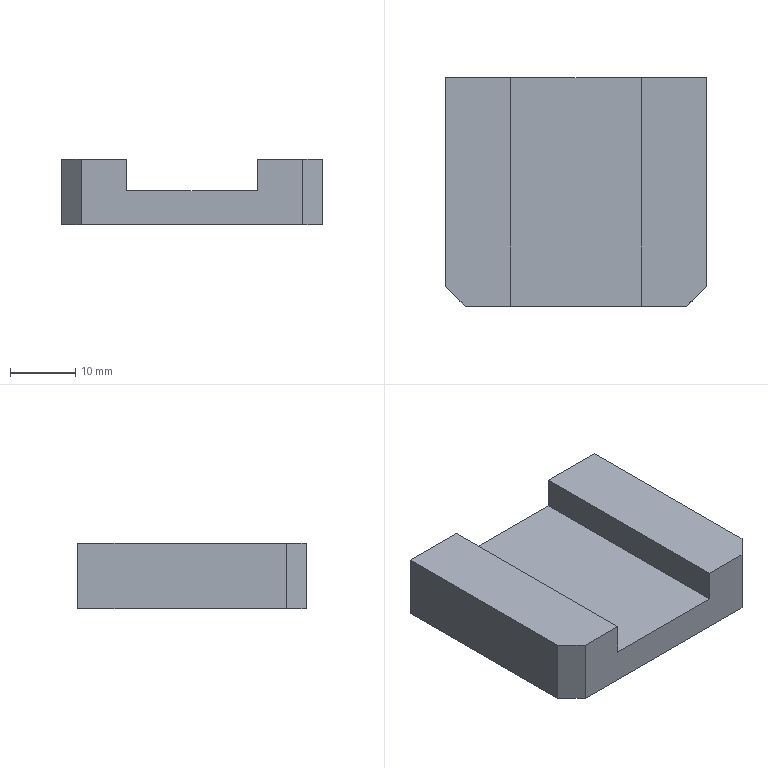Part | STEP file | PN_0017 | 1 solid | 12 faces | box 40 x 35 x 10 mm | volume 10550 mm3 | plane 12
STEP:
#1=CARTESIAN_POINT('',(0.,0.,0.));
#2=DIRECTION('',(0.,0.,1.));
#3=DIRECTION('',(1.,0.,0.));
#4=AXIS2_PLACEMENT_3D('',#1,#2,#3);
#5=CARTESIAN_POINT('',(10.,-17.5,10.));
#6=VERTEX_POINT('',#5);
#7=CARTESIAN_POINT('',(17.,-17.5,10.));
#8=VERTEX_POINT('',#7);
#9=CARTESIAN_POINT('',(-20.,-17.5,10.));
#10=DIRECTION('',(1.,0.,0.));
#11=VECTOR('',#10,1.);
#12=LINE('',#9,#11);
#13=CARTESIAN_POINT('',(20.,-17.5,10.));
#14=DIRECTION('',(0.,0.,1.));
#15=DIRECTION('',(1.,0.,0.));
#16=AXIS2_PLACEMENT_3D('',#13,#14,#15);
#17=PLANE('',#16);
#18=CARTESIAN_POINT('',(-40.,0.));
#19=DIRECTION('',(1.,0.));
#20=VECTOR('',#19,1.);
#21=LINE('',#18,#20);
#22=(GEOMETRIC_REPRESENTATION_CONTEXT(2)PARAMETRIC_REPRESENTATION_CONTEXT()REPRESENTATION_CONTEXT('',''));
#23=DEFINITIONAL_REPRESENTATION('',(#21),#22);
#24=PCURVE('',#17,#23);
#25=CARTESIAN_POINT('',(-20.,-17.5,10.));
#26=DIRECTION('',(0.,1.,0.));
#27=DIRECTION('',(0.,0.,1.));
#28=AXIS2_PLACEMENT_3D('',#25,#26,#27);
#29=PLANE('',#28);
#30=CARTESIAN_POINT('',(0.,0.));
#31=DIRECTION('',(0.,1.));
#32=VECTOR('',#31,1.);
#33=LINE('',#30,#32);
#34=(GEOMETRIC_REPRESENTATION_CONTEXT(2)PARAMETRIC_REPRESENTATION_CONTEXT()REPRESENTATION_CONTEXT('',''));
#35=DEFINITIONAL_REPRESENTATION('',(#33),#34);
#36=PCURVE('',#29,#35);
#37=SURFACE_CURVE('',#12,(#24,#36),.PCURVE_S1.);
#38=EDGE_CURVE('',#6,#8,#37,.T.);
#39=ORIENTED_EDGE('',*,*,#38,.T.);
#40=CARTESIAN_POINT('',(20.,-14.5,10.));
#41=VERTEX_POINT('',#40);
#42=CARTESIAN_POINT('',(18.5,-16.,10.));
#43=DIRECTION('',(0.7071,0.7071,0.));
#44=VECTOR('',#43,1.);
#45=LINE('',#42,#44);
#46=CARTESIAN_POINT('',(-1.5,1.5));
#47=DIRECTION('',(0.7071,0.7071));
#48=VECTOR('',#47,1.);
#49=LINE('',#46,#48);
#50=(GEOMETRIC_REPRESENTATION_CONTEXT(2)PARAMETRIC_REPRESENTATION_CONTEXT()REPRESENTATION_CONTEXT('',''));
#51=DEFINITIONAL_REPRESENTATION('',(#49),#50);
#52=PCURVE('',#17,#51);
#53=CARTESIAN_POINT('',(20.,-14.5,10.));
#54=DIRECTION('',(-0.7071,0.7071,0.));
#55=DIRECTION('',(-0.7071,-0.7071,0.));
#56=AXIS2_PLACEMENT_3D('',#53,#54,#55);
#57=PLANE('',#56);
#58=CARTESIAN_POINT('',(2.121,0.));
#59=DIRECTION('',(-1.,0.));
#60=VECTOR('',#59,1.);
#61=LINE('',#58,#60);
#62=(GEOMETRIC_REPRESENTATION_CONTEXT(2)PARAMETRIC_REPRESENTATION_CONTEXT()REPRESENTATION_CONTEXT('',''));
#63=DEFINITIONAL_REPRESENTATION('',(#61),#62);
#64=PCURVE('',#57,#63);
#65=SURFACE_CURVE('',#45,(#52,#64),.PCURVE_S1.);
#66=EDGE_CURVE('',#8,#41,#65,.T.);
#67=ORIENTED_EDGE('',*,*,#66,.T.);
#68=CARTESIAN_POINT('',(20.,17.5,10.));
#69=VERTEX_POINT('',#68);
#70=CARTESIAN_POINT('',(20.,17.5,10.));
#71=DIRECTION('',(0.,1.,0.));
#72=VECTOR('',#71,1.);
#73=LINE('',#70,#72);
#74=CARTESIAN_POINT('',(0.,35.));
#75=DIRECTION('',(0.,1.));
#76=VECTOR('',#75,1.);
#77=LINE('',#74,#76);
#78=(GEOMETRIC_REPRESENTATION_CONTEXT(2)PARAMETRIC_REPRESENTATION_CONTEXT()REPRESENTATION_CONTEXT('',''));
#79=DEFINITIONAL_REPRESENTATION('',(#77),#78);
#80=PCURVE('',#17,#79);
#81=CARTESIAN_POINT('',(20.,17.5,10.));
#82=DIRECTION('',(-1.,0.,0.));
#83=DIRECTION('',(0.,-1.,0.));
#84=AXIS2_PLACEMENT_3D('',#81,#82,#83);
#85=PLANE('',#84);
#86=CARTESIAN_POINT('',(0.,0.));
#87=DIRECTION('',(-1.,0.));
#88=VECTOR('',#87,1.);
#89=LINE('',#86,#88);
#90=(GEOMETRIC_REPRESENTATION_CONTEXT(2)PARAMETRIC_REPRESENTATION_CONTEXT()REPRESENTATION_CONTEXT('',''));
#91=DEFINITIONAL_REPRESENTATION('',(#89),#90);
#92=PCURVE('',#85,#91);
#93=SURFACE_CURVE('',#73,(#80,#92),.PCURVE_S1.);
#94=EDGE_CURVE('',#41,#69,#93,.T.);
#95=ORIENTED_EDGE('',*,*,#94,.T.);
#96=CARTESIAN_POINT('',(10.,17.5,10.));
#97=VERTEX_POINT('',#96);
#98=CARTESIAN_POINT('',(-20.,17.5,10.));
#99=DIRECTION('',(-1.,0.,0.));
#100=VECTOR('',#99,1.);
#101=LINE('',#98,#100);
#102=CARTESIAN_POINT('',(-40.,35.));
#103=DIRECTION('',(-1.,0.));
#104=VECTOR('',#103,1.);
#105=LINE('',#102,#104);
#106=(GEOMETRIC_REPRESENTATION_CONTEXT(2)PARAMETRIC_REPRESENTATION_CONTEXT()REPRESENTATION_CONTEXT('',''));
#107=DEFINITIONAL_REPRESENTATION('',(#105),#106);
#108=PCURVE('',#17,#107);
#109=CARTESIAN_POINT('',(-20.,17.5,10.));
#110=DIRECTION('',(0.,-1.,0.));
#111=DIRECTION('',(0.,0.,-1.));
#112=AXIS2_PLACEMENT_3D('',#109,#110,#111);
#113=PLANE('',#112);
#114=CARTESIAN_POINT('',(0.,0.));
#115=DIRECTION('',(0.,-1.));
#116=VECTOR('',#115,1.);
#117=LINE('',#114,#116);
#118=(GEOMETRIC_REPRESENTATION_CONTEXT(2)PARAMETRIC_REPRESENTATION_CONTEXT()REPRESENTATION_CONTEXT('',''));
#119=DEFINITIONAL_REPRESENTATION('',(#117),#118);
#120=PCURVE('',#113,#119);
#121=SURFACE_CURVE('',#101,(#108,#120),.PCURVE_S1.);
#122=EDGE_CURVE('',#69,#97,#121,.T.);
#123=ORIENTED_EDGE('',*,*,#122,.T.);
#124=CARTESIAN_POINT('',(10.,17.5,10.));
#125=DIRECTION('',(0.,1.,0.));
#126=VECTOR('',#125,1.);
#127=LINE('',#124,#126);
#128=CARTESIAN_POINT('',(-10.,35.));
#129=DIRECTION('',(0.,1.));
#130=VECTOR('',#129,1.);
#131=LINE('',#128,#130);
#132=(GEOMETRIC_REPRESENTATION_CONTEXT(2)PARAMETRIC_REPRESENTATION_CONTEXT()REPRESENTATION_CONTEXT('',''));
#133=DEFINITIONAL_REPRESENTATION('',(#131),#132);
#134=PCURVE('',#17,#133);
#135=CARTESIAN_POINT('',(10.,17.5,5.2));
#136=DIRECTION('',(1.,0.,0.));
#137=DIRECTION('',(0.,0.,-1.));
#138=AXIS2_PLACEMENT_3D('',#135,#136,#137);
#139=PLANE('',#138);
#140=CARTESIAN_POINT('',(-4.8,0.));
#141=DIRECTION('',(0.,1.));
#142=VECTOR('',#141,1.);
#143=LINE('',#140,#142);
#144=(GEOMETRIC_REPRESENTATION_CONTEXT(2)PARAMETRIC_REPRESENTATION_CONTEXT()REPRESENTATION_CONTEXT('',''));
#145=DEFINITIONAL_REPRESENTATION('',(#143),#144);
#146=PCURVE('',#139,#145);
#147=SURFACE_CURVE('',#127,(#134,#146),.PCURVE_S1.);
#148=EDGE_CURVE('',#6,#97,#147,.T.);
#149=ORIENTED_EDGE('',*,*,#148,.F.);
#150=EDGE_LOOP('',(#39,#67,#95,#123,#149));
#151=FACE_BOUND('',#150,.T.);
#152=ADVANCED_FACE('',(#151),#17,.T.);
#153=ORIENTED_EDGE('',*,*,#94,.F.);
#154=CARTESIAN_POINT('',(20.,-14.5,0.));
#155=VERTEX_POINT('',#154);
#156=CARTESIAN_POINT('',(20.,-14.5,10.));
#157=DIRECTION('',(0.,0.,-1.));
#158=VECTOR('',#157,1.);
#159=LINE('',#156,#158);
#160=CARTESIAN_POINT('',(32.,0.));
#161=DIRECTION('',(0.,-1.));
#162=VECTOR('',#161,1.);
#163=LINE('',#160,#162);
#164=(GEOMETRIC_REPRESENTATION_CONTEXT(2)PARAMETRIC_REPRESENTATION_CONTEXT()REPRESENTATION_CONTEXT('',''));
#165=DEFINITIONAL_REPRESENTATION('',(#163),#164);
#166=PCURVE('',#85,#165);
#167=CARTESIAN_POINT('',(0.,0.));
#168=DIRECTION('',(0.,-1.));
#169=VECTOR('',#168,1.);
#170=LINE('',#167,#169);
#171=(GEOMETRIC_REPRESENTATION_CONTEXT(2)PARAMETRIC_REPRESENTATION_CONTEXT()REPRESENTATION_CONTEXT('',''));
#172=DEFINITIONAL_REPRESENTATION('',(#170),#171);
#173=PCURVE('',#57,#172);
#174=SURFACE_CURVE('',#159,(#166,#173),.PCURVE_S1.);
#175=EDGE_CURVE('',#41,#155,#174,.T.);
#176=ORIENTED_EDGE('',*,*,#175,.T.);
#177=CARTESIAN_POINT('',(20.,17.5,0.));
#178=VERTEX_POINT('',#177);
#179=CARTESIAN_POINT('',(20.,17.5,0.));
#180=DIRECTION('',(0.,1.,0.));
#181=VECTOR('',#180,1.);
#182=LINE('',#179,#181);
#183=CARTESIAN_POINT('',(0.,-10.));
#184=DIRECTION('',(-1.,0.));
#185=VECTOR('',#184,1.);
#186=LINE('',#183,#185);
#187=(GEOMETRIC_REPRESENTATION_CONTEXT(2)PARAMETRIC_REPRESENTATION_CONTEXT()REPRESENTATION_CONTEXT('',''));
#188=DEFINITIONAL_REPRESENTATION('',(#186),#187);
#189=PCURVE('',#85,#188);
#190=CARTESIAN_POINT('',(20.,-17.5,0.));
#191=DIRECTION('',(0.,0.,1.));
#192=DIRECTION('',(1.,0.,0.));
#193=AXIS2_PLACEMENT_3D('',#190,#191,#192);
#194=PLANE('',#193);
#195=CARTESIAN_POINT('',(0.,35.));
#196=DIRECTION('',(0.,1.));
#197=VECTOR('',#196,1.);
#198=LINE('',#195,#197);
#199=(GEOMETRIC_REPRESENTATION_CONTEXT(2)PARAMETRIC_REPRESENTATION_CONTEXT()REPRESENTATION_CONTEXT('',''));
#200=DEFINITIONAL_REPRESENTATION('',(#198),#199);
#201=PCURVE('',#194,#200);
#202=SURFACE_CURVE('',#182,(#189,#201),.PCURVE_S1.);
#203=EDGE_CURVE('',#155,#178,#202,.T.);
#204=ORIENTED_EDGE('',*,*,#203,.T.);
#205=CARTESIAN_POINT('',(20.,17.5,10.));
#206=DIRECTION('',(0.,0.,-1.));
#207=VECTOR('',#206,1.);
#208=LINE('',#205,#207);
#209=CARTESIAN_POINT('',(0.,0.));
#210=DIRECTION('',(0.,-1.));
#211=VECTOR('',#210,1.);
#212=LINE('',#209,#211);
#213=(GEOMETRIC_REPRESENTATION_CONTEXT(2)PARAMETRIC_REPRESENTATION_CONTEXT()REPRESENTATION_CONTEXT('',''));
#214=DEFINITIONAL_REPRESENTATION('',(#212),#213);
#215=PCURVE('',#85,#214);
#216=CARTESIAN_POINT('',(0.,40.));
#217=DIRECTION('',(1.,0.));
#218=VECTOR('',#217,1.);
#219=LINE('',#216,#218);
#220=(GEOMETRIC_REPRESENTATION_CONTEXT(2)PARAMETRIC_REPRESENTATION_CONTEXT()REPRESENTATION_CONTEXT('',''));
#221=DEFINITIONAL_REPRESENTATION('',(#219),#220);
#222=PCURVE('',#113,#221);
#223=SURFACE_CURVE('',#208,(#215,#222),.PCURVE_S1.);
#224=EDGE_CURVE('',#69,#178,#223,.T.);
#225=ORIENTED_EDGE('',*,*,#224,.F.);
#226=EDGE_LOOP('',(#153,#176,#204,#225));
#227=FACE_BOUND('',#226,.T.);
#228=ADVANCED_FACE('',(#227),#85,.F.);
#229=CARTESIAN_POINT('',(10.,17.5,5.2));
#230=VERTEX_POINT('',#229);
#231=CARTESIAN_POINT('',(-10.,17.5,5.2));
#232=VERTEX_POINT('',#231);
#233=CARTESIAN_POINT('',(-10.,17.5,5.2));
#234=DIRECTION('',(-1.,0.,0.));
#235=VECTOR('',#234,1.);
#236=LINE('',#233,#235);
#237=CARTESIAN_POINT('',(4.8,10.));
#238=DIRECTION('',(0.,-1.));
#239=VECTOR('',#238,1.);
#240=LINE('',#237,#239);
#241=(GEOMETRIC_REPRESENTATION_CONTEXT(2)PARAMETRIC_REPRESENTATION_CONTEXT()REPRESENTATION_CONTEXT('',''));
#242=DEFINITIONAL_REPRESENTATION('',(#240),#241);
#243=PCURVE('',#113,#242);
#244=CARTESIAN_POINT('',(10.,-17.5,5.2));
#245=DIRECTION('',(0.,0.,1.));
#246=DIRECTION('',(1.,0.,0.));
#247=AXIS2_PLACEMENT_3D('',#244,#245,#246);
#248=PLANE('',#247);
#249=CARTESIAN_POINT('',(-20.,35.));
#250=DIRECTION('',(-1.,0.));
#251=VECTOR('',#250,1.);
#252=LINE('',#249,#251);
#253=(GEOMETRIC_REPRESENTATION_CONTEXT(2)PARAMETRIC_REPRESENTATION_CONTEXT()REPRESENTATION_CONTEXT('',''));
#254=DEFINITIONAL_REPRESENTATION('',(#252),#253);
#255=PCURVE('',#248,#254);
#256=SURFACE_CURVE('',#236,(#243,#255),.PCURVE_S1.);
#257=EDGE_CURVE('',#230,#232,#256,.T.);
#258=ORIENTED_EDGE('',*,*,#257,.F.);
#259=CARTESIAN_POINT('',(10.,17.5,5.2));
#260=DIRECTION('',(0.,0.,1.));
#261=VECTOR('',#260,1.);
#262=LINE('',#259,#261);
#263=CARTESIAN_POINT('',(4.8,30.));
#264=DIRECTION('',(-1.,0.));
#265=VECTOR('',#264,1.);
#266=LINE('',#263,#265);
#267=(GEOMETRIC_REPRESENTATION_CONTEXT(2)PARAMETRIC_REPRESENTATION_CONTEXT()REPRESENTATION_CONTEXT('',''));
#268=DEFINITIONAL_REPRESENTATION('',(#266),#267);
#269=PCURVE('',#113,#268);
#270=CARTESIAN_POINT('',(0.,0.));
#271=DIRECTION('',(-1.,0.));
#272=VECTOR('',#271,1.);
#273=LINE('',#270,#272);
#274=(GEOMETRIC_REPRESENTATION_CONTEXT(2)PARAMETRIC_REPRESENTATION_CONTEXT()REPRESENTATION_CONTEXT('',''));
#275=DEFINITIONAL_REPRESENTATION('',(#273),#274);
#276=PCURVE('',#139,#275);
#277=SURFACE_CURVE('',#262,(#269,#276),.PCURVE_S1.);
#278=EDGE_CURVE('',#230,#97,#277,.T.);
#279=ORIENTED_EDGE('',*,*,#278,.T.);
#280=ORIENTED_EDGE('',*,*,#122,.F.);
#281=ORIENTED_EDGE('',*,*,#224,.T.);
#282=CARTESIAN_POINT('',(-20.,17.5,0.));
#283=VERTEX_POINT('',#282);
#284=CARTESIAN_POINT('',(-20.,17.5,0.));
#285=DIRECTION('',(-1.,0.,0.));
#286=VECTOR('',#285,1.);
#287=LINE('',#284,#286);
#288=CARTESIAN_POINT('',(10.,0.));
#289=DIRECTION('',(0.,-1.));
#290=VECTOR('',#289,1.);
#291=LINE('',#288,#290);
#292=(GEOMETRIC_REPRESENTATION_CONTEXT(2)PARAMETRIC_REPRESENTATION_CONTEXT()REPRESENTATION_CONTEXT('',''));
#293=DEFINITIONAL_REPRESENTATION('',(#291),#292);
#294=PCURVE('',#113,#293);
#295=CARTESIAN_POINT('',(-40.,35.));
#296=DIRECTION('',(-1.,0.));
#297=VECTOR('',#296,1.);
#298=LINE('',#295,#297);
#299=(GEOMETRIC_REPRESENTATION_CONTEXT(2)PARAMETRIC_REPRESENTATION_CONTEXT()REPRESENTATION_CONTEXT('',''));
#300=DEFINITIONAL_REPRESENTATION('',(#298),#299);
#301=PCURVE('',#194,#300);
#302=SURFACE_CURVE('',#287,(#294,#301),.PCURVE_S1.);
#303=EDGE_CURVE('',#178,#283,#302,.T.);
#304=ORIENTED_EDGE('',*,*,#303,.T.);
#305=CARTESIAN_POINT('',(-20.,17.5,10.));
#306=VERTEX_POINT('',#305);
#307=CARTESIAN_POINT('',(-20.,17.5,10.));
#308=DIRECTION('',(0.,0.,-1.));
#309=VECTOR('',#308,1.);
#310=LINE('',#307,#309);
#311=CARTESIAN_POINT('',(0.,0.));
#312=DIRECTION('',(1.,0.));
#313=VECTOR('',#312,1.);
#314=LINE('',#311,#313);
#315=(GEOMETRIC_REPRESENTATION_CONTEXT(2)PARAMETRIC_REPRESENTATION_CONTEXT()REPRESENTATION_CONTEXT('',''));
#316=DEFINITIONAL_REPRESENTATION('',(#314),#315);
#317=PCURVE('',#113,#316);
#318=CARTESIAN_POINT('',(-20.,17.5,10.));
#319=DIRECTION('',(1.,0.,0.));
#320=DIRECTION('',(0.,1.,0.));
#321=AXIS2_PLACEMENT_3D('',#318,#319,#320);
#322=PLANE('',#321);
#323=CARTESIAN_POINT('',(0.,0.));
#324=DIRECTION('',(0.,-1.));
#325=VECTOR('',#324,1.);
#326=LINE('',#323,#325);
#327=(GEOMETRIC_REPRESENTATION_CONTEXT(2)PARAMETRIC_REPRESENTATION_CONTEXT()REPRESENTATION_CONTEXT('',''));
#328=DEFINITIONAL_REPRESENTATION('',(#326),#327);
#329=PCURVE('',#322,#328);
#330=SURFACE_CURVE('',#310,(#317,#329),.PCURVE_S1.);
#331=EDGE_CURVE('',#306,#283,#330,.T.);
#332=ORIENTED_EDGE('',*,*,#331,.F.);
#333=CARTESIAN_POINT('',(-10.,17.5,10.));
#334=VERTEX_POINT('',#333);
#335=CARTESIAN_POINT('',(-20.,17.5,10.));
#336=DIRECTION('',(-1.,0.,0.));
#337=VECTOR('',#336,1.);
#338=LINE('',#335,#337);
#339=CARTESIAN_POINT('',(0.,0.));
#340=DIRECTION('',(0.,-1.));
#341=VECTOR('',#340,1.);
#342=LINE('',#339,#341);
#343=(GEOMETRIC_REPRESENTATION_CONTEXT(2)PARAMETRIC_REPRESENTATION_CONTEXT()REPRESENTATION_CONTEXT('',''));
#344=DEFINITIONAL_REPRESENTATION('',(#342),#343);
#345=PCURVE('',#113,#344);
#346=CARTESIAN_POINT('',(20.,-17.5,10.));
#347=DIRECTION('',(0.,0.,1.));
#348=DIRECTION('',(1.,0.,0.));
#349=AXIS2_PLACEMENT_3D('',#346,#347,#348);
#350=PLANE('',#349);
#351=CARTESIAN_POINT('',(-40.,35.));
#352=DIRECTION('',(-1.,0.));
#353=VECTOR('',#352,1.);
#354=LINE('',#351,#353);
#355=(GEOMETRIC_REPRESENTATION_CONTEXT(2)PARAMETRIC_REPRESENTATION_CONTEXT()REPRESENTATION_CONTEXT('',''));
#356=DEFINITIONAL_REPRESENTATION('',(#354),#355);
#357=PCURVE('',#350,#356);
#358=SURFACE_CURVE('',#338,(#345,#357),.PCURVE_S1.);
#359=EDGE_CURVE('',#334,#306,#358,.T.);
#360=ORIENTED_EDGE('',*,*,#359,.F.);
#361=CARTESIAN_POINT('',(-10.,17.5,5.2));
#362=DIRECTION('',(0.,0.,1.));
#363=VECTOR('',#362,1.);
#364=LINE('',#361,#363);
#365=CARTESIAN_POINT('',(4.8,10.));
#366=DIRECTION('',(-1.,0.));
#367=VECTOR('',#366,1.);
#368=LINE('',#365,#367);
#369=(GEOMETRIC_REPRESENTATION_CONTEXT(2)PARAMETRIC_REPRESENTATION_CONTEXT()REPRESENTATION_CONTEXT('',''));
#370=DEFINITIONAL_REPRESENTATION('',(#368),#369);
#371=PCURVE('',#113,#370);
#372=CARTESIAN_POINT('',(-10.,17.5,5.2));
#373=DIRECTION('',(-1.,0.,0.));
#374=DIRECTION('',(0.,0.,1.));
#375=AXIS2_PLACEMENT_3D('',#372,#373,#374);
#376=PLANE('',#375);
#377=CARTESIAN_POINT('',(0.,0.));
#378=DIRECTION('',(1.,0.));
#379=VECTOR('',#378,1.);
#380=LINE('',#377,#379);
#381=(GEOMETRIC_REPRESENTATION_CONTEXT(2)PARAMETRIC_REPRESENTATION_CONTEXT()REPRESENTATION_CONTEXT('',''));
#382=DEFINITIONAL_REPRESENTATION('',(#380),#381);
#383=PCURVE('',#376,#382);
#384=SURFACE_CURVE('',#364,(#371,#383),.PCURVE_S1.);
#385=EDGE_CURVE('',#232,#334,#384,.T.);
#386=ORIENTED_EDGE('',*,*,#385,.F.);
#387=EDGE_LOOP('',(#258,#279,#280,#281,#304,#332,#360,#386));
#388=FACE_BOUND('',#387,.T.);
#389=ADVANCED_FACE('',(#388),#113,.F.);
#390=CARTESIAN_POINT('',(-20.,-14.5,0.));
#391=VERTEX_POINT('',#390);
#392=CARTESIAN_POINT('',(-20.,17.5,0.));
#393=DIRECTION('',(0.,-1.,0.));
#394=VECTOR('',#393,1.);
#395=LINE('',#392,#394);
#396=CARTESIAN_POINT('',(0.,-10.));
#397=DIRECTION('',(-1.,0.));
#398=VECTOR('',#397,1.);
#399=LINE('',#396,#398);
#400=(GEOMETRIC_REPRESENTATION_CONTEXT(2)PARAMETRIC_REPRESENTATION_CONTEXT()REPRESENTATION_CONTEXT('',''));
#401=DEFINITIONAL_REPRESENTATION('',(#399),#400);
#402=PCURVE('',#322,#401);
#403=CARTESIAN_POINT('',(-40.,35.));
#404=DIRECTION('',(0.,-1.));
#405=VECTOR('',#404,1.);
#406=LINE('',#403,#405);
#407=(GEOMETRIC_REPRESENTATION_CONTEXT(2)PARAMETRIC_REPRESENTATION_CONTEXT()REPRESENTATION_CONTEXT('',''));
#408=DEFINITIONAL_REPRESENTATION('',(#406),#407);
#409=PCURVE('',#194,#408);
#410=SURFACE_CURVE('',#395,(#402,#409),.PCURVE_S1.);
#411=EDGE_CURVE('',#283,#391,#410,.T.);
#412=ORIENTED_EDGE('',*,*,#411,.T.);
#413=CARTESIAN_POINT('',(-20.,-14.5,10.));
#414=VERTEX_POINT('',#413);
#415=CARTESIAN_POINT('',(-20.,-14.5,10.));
#416=DIRECTION('',(0.,0.,1.));
#417=VECTOR('',#416,1.);
#418=LINE('',#415,#417);
#419=CARTESIAN_POINT('',(-32.,0.));
#420=DIRECTION('',(0.,1.));
#421=VECTOR('',#420,1.);
#422=LINE('',#419,#421);
#423=(GEOMETRIC_REPRESENTATION_CONTEXT(2)PARAMETRIC_REPRESENTATION_CONTEXT()REPRESENTATION_CONTEXT('',''));
#424=DEFINITIONAL_REPRESENTATION('',(#422),#423);
#425=PCURVE('',#322,#424);
#426=CARTESIAN_POINT('',(-17.,-17.5,10.));
#427=DIRECTION('',(0.7071,0.7071,0.));
#428=DIRECTION('',(-0.7071,0.7071,0.));
#429=AXIS2_PLACEMENT_3D('',#426,#427,#428);
#430=PLANE('',#429);
#431=CARTESIAN_POINT('',(4.243,0.));
#432=DIRECTION('',(0.,1.));
#433=VECTOR('',#432,1.);
#434=LINE('',#431,#433);
#435=(GEOMETRIC_REPRESENTATION_CONTEXT(2)PARAMETRIC_REPRESENTATION_CONTEXT()REPRESENTATION_CONTEXT('',''));
#436=DEFINITIONAL_REPRESENTATION('',(#434),#435);
#437=PCURVE('',#430,#436);
#438=SURFACE_CURVE('',#418,(#425,#437),.PCURVE_S1.);
#439=EDGE_CURVE('',#391,#414,#438,.T.);
#440=ORIENTED_EDGE('',*,*,#439,.T.);
#441=CARTESIAN_POINT('',(-20.,17.5,10.));
#442=DIRECTION('',(0.,-1.,0.));
#443=VECTOR('',#442,1.);
#444=LINE('',#441,#443);
#445=CARTESIAN_POINT('',(0.,0.));
#446=DIRECTION('',(-1.,0.));
#447=VECTOR('',#446,1.);
#448=LINE('',#445,#447);
#449=(GEOMETRIC_REPRESENTATION_CONTEXT(2)PARAMETRIC_REPRESENTATION_CONTEXT()REPRESENTATION_CONTEXT('',''));
#450=DEFINITIONAL_REPRESENTATION('',(#448),#449);
#451=PCURVE('',#322,#450);
#452=CARTESIAN_POINT('',(-40.,35.));
#453=DIRECTION('',(0.,-1.));
#454=VECTOR('',#453,1.);
#455=LINE('',#452,#454);
#456=(GEOMETRIC_REPRESENTATION_CONTEXT(2)PARAMETRIC_REPRESENTATION_CONTEXT()REPRESENTATION_CONTEXT('',''));
#457=DEFINITIONAL_REPRESENTATION('',(#455),#456);
#458=PCURVE('',#350,#457);
#459=SURFACE_CURVE('',#444,(#451,#458),.PCURVE_S1.);
#460=EDGE_CURVE('',#306,#414,#459,.T.);
#461=ORIENTED_EDGE('',*,*,#460,.F.);
#462=ORIENTED_EDGE('',*,*,#331,.T.);
#463=EDGE_LOOP('',(#412,#440,#461,#462));
#464=FACE_BOUND('',#463,.T.);
#465=ADVANCED_FACE('',(#464),#322,.F.);
#466=CARTESIAN_POINT('',(-17.,-17.5,10.));
#467=VERTEX_POINT('',#466);
#468=CARTESIAN_POINT('',(-10.,-17.5,10.));
#469=VERTEX_POINT('',#468);
#470=CARTESIAN_POINT('',(-20.,-17.5,10.));
#471=DIRECTION('',(1.,0.,0.));
#472=VECTOR('',#471,1.);
#473=LINE('',#470,#472);
#474=CARTESIAN_POINT('',(0.,0.));
#475=DIRECTION('',(0.,1.));
#476=VECTOR('',#475,1.);
#477=LINE('',#474,#476);
#478=(GEOMETRIC_REPRESENTATION_CONTEXT(2)PARAMETRIC_REPRESENTATION_CONTEXT()REPRESENTATION_CONTEXT('',''));
#479=DEFINITIONAL_REPRESENTATION('',(#477),#478);
#480=PCURVE('',#29,#479);
#481=CARTESIAN_POINT('',(-40.,0.));
#482=DIRECTION('',(1.,0.));
#483=VECTOR('',#482,1.);
#484=LINE('',#481,#483);
#485=(GEOMETRIC_REPRESENTATION_CONTEXT(2)PARAMETRIC_REPRESENTATION_CONTEXT()REPRESENTATION_CONTEXT('',''));
#486=DEFINITIONAL_REPRESENTATION('',(#484),#485);
#487=PCURVE('',#350,#486);
#488=SURFACE_CURVE('',#473,(#480,#487),.PCURVE_S1.);
#489=EDGE_CURVE('',#467,#469,#488,.T.);
#490=ORIENTED_EDGE('',*,*,#489,.F.);
#491=CARTESIAN_POINT('',(-17.,-17.5,0.));
#492=VERTEX_POINT('',#491);
#493=CARTESIAN_POINT('',(-17.,-17.5,10.));
#494=DIRECTION('',(0.,0.,-1.));
#495=VECTOR('',#494,1.);
#496=LINE('',#493,#495);
#497=CARTESIAN_POINT('',(0.,3.));
#498=DIRECTION('',(-1.,0.));
#499=VECTOR('',#498,1.);
#500=LINE('',#497,#499);
#501=(GEOMETRIC_REPRESENTATION_CONTEXT(2)PARAMETRIC_REPRESENTATION_CONTEXT()REPRESENTATION_CONTEXT('',''));
#502=DEFINITIONAL_REPRESENTATION('',(#500),#501);
#503=PCURVE('',#29,#502);
#504=CARTESIAN_POINT('',(0.,0.));
#505=DIRECTION('',(0.,-1.));
#506=VECTOR('',#505,1.);
#507=LINE('',#504,#506);
#508=(GEOMETRIC_REPRESENTATION_CONTEXT(2)PARAMETRIC_REPRESENTATION_CONTEXT()REPRESENTATION_CONTEXT('',''));
#509=DEFINITIONAL_REPRESENTATION('',(#507),#508);
#510=PCURVE('',#430,#509);
#511=SURFACE_CURVE('',#496,(#503,#510),.PCURVE_S1.);
#512=EDGE_CURVE('',#467,#492,#511,.T.);
#513=ORIENTED_EDGE('',*,*,#512,.T.);
#514=CARTESIAN_POINT('',(17.,-17.5,0.));
#515=VERTEX_POINT('',#514);
#516=CARTESIAN_POINT('',(-20.,-17.5,0.));
#517=DIRECTION('',(1.,0.,0.));
#518=VECTOR('',#517,1.);
#519=LINE('',#516,#518);
#520=CARTESIAN_POINT('',(-10.,0.));
#521=DIRECTION('',(0.,1.));
#522=VECTOR('',#521,1.);
#523=LINE('',#520,#522);
#524=(GEOMETRIC_REPRESENTATION_CONTEXT(2)PARAMETRIC_REPRESENTATION_CONTEXT()REPRESENTATION_CONTEXT('',''));
#525=DEFINITIONAL_REPRESENTATION('',(#523),#524);
#526=PCURVE('',#29,#525);
#527=CARTESIAN_POINT('',(-40.,0.));
#528=DIRECTION('',(1.,0.));
#529=VECTOR('',#528,1.);
#530=LINE('',#527,#529);
#531=(GEOMETRIC_REPRESENTATION_CONTEXT(2)PARAMETRIC_REPRESENTATION_CONTEXT()REPRESENTATION_CONTEXT('',''));
#532=DEFINITIONAL_REPRESENTATION('',(#530),#531);
#533=PCURVE('',#194,#532);
#534=SURFACE_CURVE('',#519,(#526,#533),.PCURVE_S1.);
#535=EDGE_CURVE('',#492,#515,#534,.T.);
#536=ORIENTED_EDGE('',*,*,#535,.T.);
#537=CARTESIAN_POINT('',(17.,-17.5,10.));
#538=DIRECTION('',(0.,0.,1.));
#539=VECTOR('',#538,1.);
#540=LINE('',#537,#539);
#541=CARTESIAN_POINT('',(0.,37.));
#542=DIRECTION('',(1.,0.));
#543=VECTOR('',#542,1.);
#544=LINE('',#541,#543);
#545=(GEOMETRIC_REPRESENTATION_CONTEXT(2)PARAMETRIC_REPRESENTATION_CONTEXT()REPRESENTATION_CONTEXT('',''));
#546=DEFINITIONAL_REPRESENTATION('',(#544),#545);
#547=PCURVE('',#29,#546);
#548=CARTESIAN_POINT('',(4.243,0.));
#549=DIRECTION('',(0.,1.));
#550=VECTOR('',#549,1.);
#551=LINE('',#548,#550);
#552=(GEOMETRIC_REPRESENTATION_CONTEXT(2)PARAMETRIC_REPRESENTATION_CONTEXT()REPRESENTATION_CONTEXT('',''));
#553=DEFINITIONAL_REPRESENTATION('',(#551),#552);
#554=PCURVE('',#57,#553);
#555=SURFACE_CURVE('',#540,(#547,#554),.PCURVE_S1.);
#556=EDGE_CURVE('',#515,#8,#555,.T.);
#557=ORIENTED_EDGE('',*,*,#556,.T.);
#558=ORIENTED_EDGE('',*,*,#38,.F.);
#559=CARTESIAN_POINT('',(10.,-17.5,5.2));
#560=VERTEX_POINT('',#559);
#561=CARTESIAN_POINT('',(10.,-17.5,5.2));
#562=DIRECTION('',(0.,0.,1.));
#563=VECTOR('',#562,1.);
#564=LINE('',#561,#563);
#565=CARTESIAN_POINT('',(-4.8,30.));
#566=DIRECTION('',(1.,0.));
#567=VECTOR('',#566,1.);
#568=LINE('',#565,#567);
#569=(GEOMETRIC_REPRESENTATION_CONTEXT(2)PARAMETRIC_REPRESENTATION_CONTEXT()REPRESENTATION_CONTEXT('',''));
#570=DEFINITIONAL_REPRESENTATION('',(#568),#569);
#571=PCURVE('',#29,#570);
#572=CARTESIAN_POINT('',(0.,-35.));
#573=DIRECTION('',(-1.,0.));
#574=VECTOR('',#573,1.);
#575=LINE('',#572,#574);
#576=(GEOMETRIC_REPRESENTATION_CONTEXT(2)PARAMETRIC_REPRESENTATION_CONTEXT()REPRESENTATION_CONTEXT('',''));
#577=DEFINITIONAL_REPRESENTATION('',(#575),#576);
#578=PCURVE('',#139,#577);
#579=SURFACE_CURVE('',#564,(#571,#578),.PCURVE_S1.);
#580=EDGE_CURVE('',#560,#6,#579,.T.);
#581=ORIENTED_EDGE('',*,*,#580,.F.);
#582=CARTESIAN_POINT('',(-10.,-17.5,5.2));
#583=VERTEX_POINT('',#582);
#584=CARTESIAN_POINT('',(-10.,-17.5,5.2));
#585=DIRECTION('',(1.,0.,0.));
#586=VECTOR('',#585,1.);
#587=LINE('',#584,#586);
#588=CARTESIAN_POINT('',(-4.8,10.));
#589=DIRECTION('',(0.,1.));
#590=VECTOR('',#589,1.);
#591=LINE('',#588,#590);
#592=(GEOMETRIC_REPRESENTATION_CONTEXT(2)PARAMETRIC_REPRESENTATION_CONTEXT()REPRESENTATION_CONTEXT('',''));
#593=DEFINITIONAL_REPRESENTATION('',(#591),#592);
#594=PCURVE('',#29,#593);
#595=CARTESIAN_POINT('',(-20.,0.));
#596=DIRECTION('',(1.,0.));
#597=VECTOR('',#596,1.);
#598=LINE('',#595,#597);
#599=(GEOMETRIC_REPRESENTATION_CONTEXT(2)PARAMETRIC_REPRESENTATION_CONTEXT()REPRESENTATION_CONTEXT('',''));
#600=DEFINITIONAL_REPRESENTATION('',(#598),#599);
#601=PCURVE('',#248,#600);
#602=SURFACE_CURVE('',#587,(#594,#601),.PCURVE_S1.);
#603=EDGE_CURVE('',#583,#560,#602,.T.);
#604=ORIENTED_EDGE('',*,*,#603,.F.);
#605=CARTESIAN_POINT('',(-10.,-17.5,5.2));
#606=DIRECTION('',(0.,0.,1.));
#607=VECTOR('',#606,1.);
#608=LINE('',#605,#607);
#609=CARTESIAN_POINT('',(-4.8,10.));
#610=DIRECTION('',(1.,0.));
#611=VECTOR('',#610,1.);
#612=LINE('',#609,#611);
#613=(GEOMETRIC_REPRESENTATION_CONTEXT(2)PARAMETRIC_REPRESENTATION_CONTEXT()REPRESENTATION_CONTEXT('',''));
#614=DEFINITIONAL_REPRESENTATION('',(#612),#613);
#615=PCURVE('',#29,#614);
#616=CARTESIAN_POINT('',(0.,-35.));
#617=DIRECTION('',(1.,0.));
#618=VECTOR('',#617,1.);
#619=LINE('',#616,#618);
#620=(GEOMETRIC_REPRESENTATION_CONTEXT(2)PARAMETRIC_REPRESENTATION_CONTEXT()REPRESENTATION_CONTEXT('',''));
#621=DEFINITIONAL_REPRESENTATION('',(#619),#620);
#622=PCURVE('',#376,#621);
#623=SURFACE_CURVE('',#608,(#615,#622),.PCURVE_S1.);
#624=EDGE_CURVE('',#583,#469,#623,.T.);
#625=ORIENTED_EDGE('',*,*,#624,.T.);
#626=EDGE_LOOP('',(#490,#513,#536,#557,#558,#581,#604,#625));
#627=FACE_BOUND('',#626,.T.);
#628=ADVANCED_FACE('',(#627),#29,.F.);
#629=ORIENTED_EDGE('',*,*,#460,.T.);
#630=CARTESIAN_POINT('',(1.5,-36.,10.));
#631=DIRECTION('',(0.7071,-0.7071,0.));
#632=VECTOR('',#631,1.);
#633=LINE('',#630,#632);
#634=CARTESIAN_POINT('',(-18.5,-18.5));
#635=DIRECTION('',(0.7071,-0.7071));
#636=VECTOR('',#635,1.);
#637=LINE('',#634,#636);
#638=(GEOMETRIC_REPRESENTATION_CONTEXT(2)PARAMETRIC_REPRESENTATION_CONTEXT()REPRESENTATION_CONTEXT('',''));
#639=DEFINITIONAL_REPRESENTATION('',(#637),#638);
#640=PCURVE('',#350,#639);
#641=CARTESIAN_POINT('',(-26.163,0.));
#642=DIRECTION('',(-1.,0.));
#643=VECTOR('',#642,1.);
#644=LINE('',#641,#643);
#645=(GEOMETRIC_REPRESENTATION_CONTEXT(2)PARAMETRIC_REPRESENTATION_CONTEXT()REPRESENTATION_CONTEXT('',''));
#646=DEFINITIONAL_REPRESENTATION('',(#644),#645);
#647=PCURVE('',#430,#646);
#648=SURFACE_CURVE('',#633,(#640,#647),.PCURVE_S1.);
#649=EDGE_CURVE('',#414,#467,#648,.T.);
#650=ORIENTED_EDGE('',*,*,#649,.T.);
#651=ORIENTED_EDGE('',*,*,#489,.T.);
#652=CARTESIAN_POINT('',(-10.,17.5,10.));
#653=DIRECTION('',(0.,-1.,0.));
#654=VECTOR('',#653,1.);
#655=LINE('',#652,#654);
#656=CARTESIAN_POINT('',(-30.,35.));
#657=DIRECTION('',(0.,-1.));
#658=VECTOR('',#657,1.);
#659=LINE('',#656,#658);
#660=(GEOMETRIC_REPRESENTATION_CONTEXT(2)PARAMETRIC_REPRESENTATION_CONTEXT()REPRESENTATION_CONTEXT('',''));
#661=DEFINITIONAL_REPRESENTATION('',(#659),#660);
#662=PCURVE('',#350,#661);
#663=CARTESIAN_POINT('',(4.8,0.));
#664=DIRECTION('',(0.,-1.));
#665=VECTOR('',#664,1.);
#666=LINE('',#663,#665);
#667=(GEOMETRIC_REPRESENTATION_CONTEXT(2)PARAMETRIC_REPRESENTATION_CONTEXT()REPRESENTATION_CONTEXT('',''));
#668=DEFINITIONAL_REPRESENTATION('',(#666),#667);
#669=PCURVE('',#376,#668);
#670=SURFACE_CURVE('',#655,(#662,#669),.PCURVE_S1.);
#671=EDGE_CURVE('',#334,#469,#670,.T.);
#672=ORIENTED_EDGE('',*,*,#671,.F.);
#673=ORIENTED_EDGE('',*,*,#359,.T.);
#674=EDGE_LOOP('',(#629,#650,#651,#672,#673));
#675=FACE_BOUND('',#674,.T.);
#676=ADVANCED_FACE('',(#675),#350,.T.);
#677=ORIENTED_EDGE('',*,*,#535,.F.);
#678=CARTESIAN_POINT('',(-17.,-17.5,0.));
#679=DIRECTION('',(-0.7071,0.7071,0.));
#680=VECTOR('',#679,1.);
#681=LINE('',#678,#680);
#682=CARTESIAN_POINT('',(-37.,0.));
#683=DIRECTION('',(-0.7071,0.7071));
#684=VECTOR('',#683,1.);
#685=LINE('',#682,#684);
#686=(GEOMETRIC_REPRESENTATION_CONTEXT(2)PARAMETRIC_REPRESENTATION_CONTEXT()REPRESENTATION_CONTEXT('',''));
#687=DEFINITIONAL_REPRESENTATION('',(#685),#686);
#688=PCURVE('',#194,#687);
#689=CARTESIAN_POINT('',(0.,-10.));
#690=DIRECTION('',(1.,0.));
#691=VECTOR('',#690,1.);
#692=LINE('',#689,#691);
#693=(GEOMETRIC_REPRESENTATION_CONTEXT(2)PARAMETRIC_REPRESENTATION_CONTEXT()REPRESENTATION_CONTEXT('',''));
#694=DEFINITIONAL_REPRESENTATION('',(#692),#693);
#695=PCURVE('',#430,#694);
#696=SURFACE_CURVE('',#681,(#688,#695),.PCURVE_S1.);
#697=EDGE_CURVE('',#492,#391,#696,.T.);
#698=ORIENTED_EDGE('',*,*,#697,.T.);
#699=ORIENTED_EDGE('',*,*,#411,.F.);
#700=ORIENTED_EDGE('',*,*,#303,.F.);
#701=ORIENTED_EDGE('',*,*,#203,.F.);
#702=CARTESIAN_POINT('',(20.,-14.5,0.));
#703=DIRECTION('',(-0.7071,-0.7071,0.));
#704=VECTOR('',#703,1.);
#705=LINE('',#702,#704);
#706=CARTESIAN_POINT('',(0.,3.));
#707=DIRECTION('',(-0.7071,-0.7071));
#708=VECTOR('',#707,1.);
#709=LINE('',#706,#708);
#710=(GEOMETRIC_REPRESENTATION_CONTEXT(2)PARAMETRIC_REPRESENTATION_CONTEXT()REPRESENTATION_CONTEXT('',''));
#711=DEFINITIONAL_REPRESENTATION('',(#709),#710);
#712=PCURVE('',#194,#711);
#713=CARTESIAN_POINT('',(0.,-10.));
#714=DIRECTION('',(1.,0.));
#715=VECTOR('',#714,1.);
#716=LINE('',#713,#715);
#717=(GEOMETRIC_REPRESENTATION_CONTEXT(2)PARAMETRIC_REPRESENTATION_CONTEXT()REPRESENTATION_CONTEXT('',''));
#718=DEFINITIONAL_REPRESENTATION('',(#716),#717);
#719=PCURVE('',#57,#718);
#720=SURFACE_CURVE('',#705,(#712,#719),.PCURVE_S1.);
#721=EDGE_CURVE('',#155,#515,#720,.T.);
#722=ORIENTED_EDGE('',*,*,#721,.T.);
#723=EDGE_LOOP('',(#677,#698,#699,#700,#701,#722));
#724=FACE_BOUND('',#723,.T.);
#725=ADVANCED_FACE('',(#724),#194,.F.);
#726=ORIENTED_EDGE('',*,*,#148,.T.);
#727=ORIENTED_EDGE('',*,*,#278,.F.);
#728=CARTESIAN_POINT('',(10.,17.5,5.2));
#729=DIRECTION('',(0.,1.,0.));
#730=VECTOR('',#729,1.);
#731=LINE('',#728,#730);
#732=CARTESIAN_POINT('',(0.,0.));
#733=DIRECTION('',(0.,1.));
#734=VECTOR('',#733,1.);
#735=LINE('',#732,#734);
#736=(GEOMETRIC_REPRESENTATION_CONTEXT(2)PARAMETRIC_REPRESENTATION_CONTEXT()REPRESENTATION_CONTEXT('',''));
#737=DEFINITIONAL_REPRESENTATION('',(#735),#736);
#738=PCURVE('',#139,#737);
#739=CARTESIAN_POINT('',(0.,35.));
#740=DIRECTION('',(0.,1.));
#741=VECTOR('',#740,1.);
#742=LINE('',#739,#741);
#743=(GEOMETRIC_REPRESENTATION_CONTEXT(2)PARAMETRIC_REPRESENTATION_CONTEXT()REPRESENTATION_CONTEXT('',''));
#744=DEFINITIONAL_REPRESENTATION('',(#742),#743);
#745=PCURVE('',#248,#744);
#746=SURFACE_CURVE('',#731,(#738,#745),.PCURVE_S1.);
#747=EDGE_CURVE('',#560,#230,#746,.T.);
#748=ORIENTED_EDGE('',*,*,#747,.F.);
#749=ORIENTED_EDGE('',*,*,#580,.T.);
#750=EDGE_LOOP('',(#726,#727,#748,#749));
#751=FACE_BOUND('',#750,.T.);
#752=ADVANCED_FACE('',(#751),#139,.F.);
#753=ORIENTED_EDGE('',*,*,#671,.T.);
#754=ORIENTED_EDGE('',*,*,#624,.F.);
#755=CARTESIAN_POINT('',(-10.,17.5,5.2));
#756=DIRECTION('',(0.,-1.,0.));
#757=VECTOR('',#756,1.);
#758=LINE('',#755,#757);
#759=CARTESIAN_POINT('',(0.,0.));
#760=DIRECTION('',(0.,-1.));
#761=VECTOR('',#760,1.);
#762=LINE('',#759,#761);
#763=(GEOMETRIC_REPRESENTATION_CONTEXT(2)PARAMETRIC_REPRESENTATION_CONTEXT()REPRESENTATION_CONTEXT('',''));
#764=DEFINITIONAL_REPRESENTATION('',(#762),#763);
#765=PCURVE('',#376,#764);
#766=CARTESIAN_POINT('',(-20.,35.));
#767=DIRECTION('',(0.,-1.));
#768=VECTOR('',#767,1.);
#769=LINE('',#766,#768);
#770=(GEOMETRIC_REPRESENTATION_CONTEXT(2)PARAMETRIC_REPRESENTATION_CONTEXT()REPRESENTATION_CONTEXT('',''));
#771=DEFINITIONAL_REPRESENTATION('',(#769),#770);
#772=PCURVE('',#248,#771);
#773=SURFACE_CURVE('',#758,(#765,#772),.PCURVE_S1.);
#774=EDGE_CURVE('',#232,#583,#773,.T.);
#775=ORIENTED_EDGE('',*,*,#774,.F.);
#776=ORIENTED_EDGE('',*,*,#385,.T.);
#777=EDGE_LOOP('',(#753,#754,#775,#776));
#778=FACE_BOUND('',#777,.T.);
#779=ADVANCED_FACE('',(#778),#376,.F.);
#780=ORIENTED_EDGE('',*,*,#747,.T.);
#781=ORIENTED_EDGE('',*,*,#257,.T.);
#782=ORIENTED_EDGE('',*,*,#774,.T.);
#783=ORIENTED_EDGE('',*,*,#603,.T.);
#784=EDGE_LOOP('',(#780,#781,#782,#783));
#785=FACE_BOUND('',#784,.T.);
#786=ADVANCED_FACE('',(#785),#248,.T.);
#787=ORIENTED_EDGE('',*,*,#649,.F.);
#788=ORIENTED_EDGE('',*,*,#439,.F.);
#789=ORIENTED_EDGE('',*,*,#697,.F.);
#790=ORIENTED_EDGE('',*,*,#512,.F.);
#791=EDGE_LOOP('',(#787,#788,#789,#790));
#792=FACE_BOUND('',#791,.T.);
#793=ADVANCED_FACE('',(#792),#430,.F.);
#794=ORIENTED_EDGE('',*,*,#66,.F.);
#795=ORIENTED_EDGE('',*,*,#556,.F.);
#796=ORIENTED_EDGE('',*,*,#721,.F.);
#797=ORIENTED_EDGE('',*,*,#175,.F.);
#798=EDGE_LOOP('',(#794,#795,#796,#797));
#799=FACE_BOUND('',#798,.T.);
#800=ADVANCED_FACE('',(#799),#57,.F.);
#801=CLOSED_SHELL('',(#152,#228,#389,#465,#628,#676,#725,#752,#779,#786,#793,#800));
#802=MANIFOLD_SOLID_BREP('',#801);
#803=(LENGTH_UNIT()NAMED_UNIT(*)SI_UNIT(.MILLI.,.METRE.));
#804=UNCERTAINTY_MEASURE_WITH_UNIT(LENGTH_MEASURE(0.0000001),#803,'','');
#805=(NAMED_UNIT(*)PLANE_ANGLE_UNIT()SI_UNIT($,.RADIAN.));
#806=(NAMED_UNIT(*)SI_UNIT($,.STERADIAN.)SOLID_ANGLE_UNIT());
#807=(GEOMETRIC_REPRESENTATION_CONTEXT(3)GLOBAL_UNCERTAINTY_ASSIGNED_CONTEXT((#804))GLOBAL_UNIT_ASSIGNED_CONTEXT((#803,#805,#806))REPRESENTATION_CONTEXT('',''));
#808=ADVANCED_BREP_SHAPE_REPRESENTATION('',(#4,#802),#807);